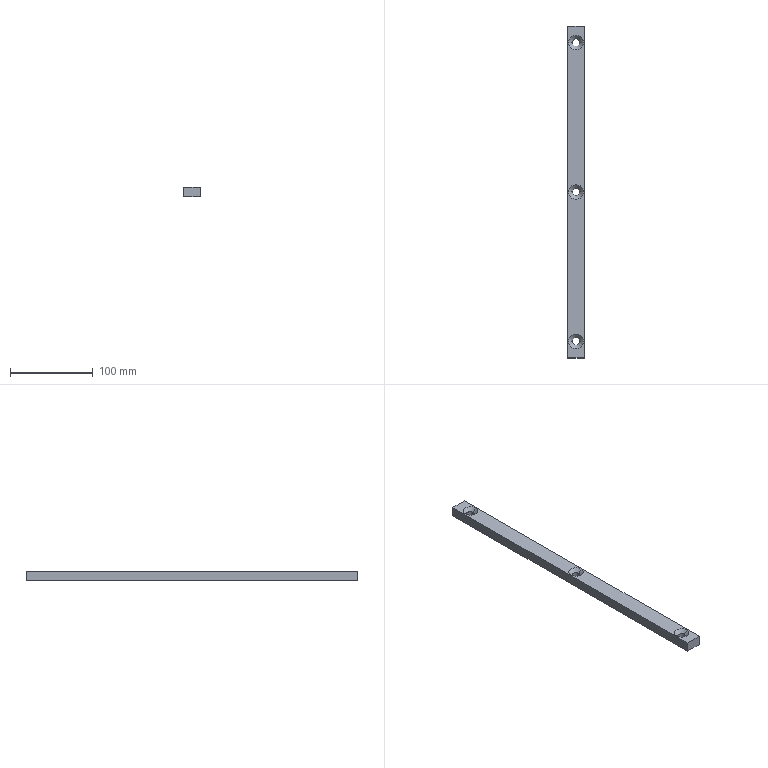Part | SolidWorks | features Extrusion 1, HoleWzd 1 | 1 solid | 18 faces | box 20 x 400 x 12 mm | volume 92676 mm3 | cone 6 | cylinder 6 | plane 6 | commonest cylinder face diameters 9 x6
STEP:
#1=CARTESIAN_POINT('',(5.5,380.,7.7));
#2=VERTEX_POINT('',#1);
#3=CARTESIAN_POINT('',(14.5,380.,7.7));
#4=VERTEX_POINT('',#3);
#5=CARTESIAN_POINT('',(10.,380.,7.7));
#6=DIRECTION('',(0.,0.,1.));
#7=DIRECTION('',(1.,0.,0.));
#8=AXIS2_PLACEMENT_3D('',#5,#6,#7);
#9=CIRCLE('',#8,4.5);
#10=EDGE_CURVE('',#2,#4,#9,.T.);
#11=ORIENTED_EDGE('',*,*,#10,.F.);
#12=CARTESIAN_POINT('',(1.2,380.,12.));
#13=VERTEX_POINT('',#12);
#14=CARTESIAN_POINT('',(1.2,380.,12.));
#15=DIRECTION('',(-0.7071,0.,0.7071));
#16=VECTOR('',#15,1000.);
#17=LINE('',#14,#16);
#18=EDGE_CURVE('',#2,#13,#17,.T.);
#19=ORIENTED_EDGE('',*,*,#18,.T.);
#20=CARTESIAN_POINT('',(18.8,380.,12.));
#21=VERTEX_POINT('',#20);
#22=CARTESIAN_POINT('',(10.,380.,12.));
#23=DIRECTION('',(0.,0.,1.));
#24=DIRECTION('',(1.,0.,0.));
#25=AXIS2_PLACEMENT_3D('',#22,#23,#24);
#26=CIRCLE('',#25,8.8);
#27=EDGE_CURVE('',#13,#21,#26,.T.);
#28=ORIENTED_EDGE('',*,*,#27,.T.);
#29=CARTESIAN_POINT('',(18.8,380.,12.));
#30=DIRECTION('',(0.7071,0.,0.7071));
#31=VECTOR('',#30,1000.);
#32=LINE('',#29,#31);
#33=EDGE_CURVE('',#4,#21,#32,.T.);
#34=ORIENTED_EDGE('',*,*,#33,.F.);
#35=EDGE_LOOP('',(#11,#19,#28,#34));
#36=FACE_OUTER_BOUND('',#35,.T.);
#37=CARTESIAN_POINT('',(10.,380.,12.));
#38=DIRECTION('',(0.,0.,1.));
#39=DIRECTION('',(1.,0.,0.));
#40=AXIS2_PLACEMENT_3D('',#37,#38,#39);
#41=CONICAL_SURFACE('',#40,8.8,0.7854);
#42=ADVANCED_FACE('',(#36),#41,.F.);
#43=CARTESIAN_POINT('',(5.5,380.,0.));
#44=VERTEX_POINT('',#43);
#45=CARTESIAN_POINT('',(14.5,380.,0.));
#46=VERTEX_POINT('',#45);
#47=CARTESIAN_POINT('',(10.,380.,0.));
#48=DIRECTION('',(0.,0.,1.));
#49=DIRECTION('',(1.,0.,0.));
#50=AXIS2_PLACEMENT_3D('',#47,#48,#49);
#51=CIRCLE('',#50,4.5);
#52=EDGE_CURVE('',#44,#46,#51,.T.);
#53=ORIENTED_EDGE('',*,*,#52,.F.);
#54=CARTESIAN_POINT('',(5.5,380.,12.));
#55=DIRECTION('',(0.,0.,1.));
#56=VECTOR('',#55,1000.);
#57=LINE('',#54,#56);
#58=EDGE_CURVE('',#44,#2,#57,.T.);
#59=ORIENTED_EDGE('',*,*,#58,.T.);
#60=ORIENTED_EDGE('',*,*,#10,.T.);
#61=CARTESIAN_POINT('',(14.5,380.,12.));
#62=DIRECTION('',(0.,0.,1.));
#63=VECTOR('',#62,1000.);
#64=LINE('',#61,#63);
#65=EDGE_CURVE('',#46,#4,#64,.T.);
#66=ORIENTED_EDGE('',*,*,#65,.F.);
#67=EDGE_LOOP('',(#53,#59,#60,#66));
#68=FACE_OUTER_BOUND('',#67,.T.);
#69=CARTESIAN_POINT('',(10.,380.,12.));
#70=DIRECTION('',(0.,0.,1.));
#71=DIRECTION('',(1.,0.,0.));
#72=AXIS2_PLACEMENT_3D('',#69,#70,#71);
#73=CYLINDRICAL_SURFACE('',#72,4.5);
#74=ADVANCED_FACE('',(#68),#73,.F.);
#75=CARTESIAN_POINT('',(5.5,200.,7.7));
#76=VERTEX_POINT('',#75);
#77=CARTESIAN_POINT('',(14.5,200.,7.7));
#78=VERTEX_POINT('',#77);
#79=CARTESIAN_POINT('',(10.,200.,7.7));
#80=DIRECTION('',(0.,0.,1.));
#81=DIRECTION('',(1.,0.,0.));
#82=AXIS2_PLACEMENT_3D('',#79,#80,#81);
#83=CIRCLE('',#82,4.5);
#84=EDGE_CURVE('',#76,#78,#83,.T.);
#85=ORIENTED_EDGE('',*,*,#84,.F.);
#86=CARTESIAN_POINT('',(1.2,200.,12.));
#87=VERTEX_POINT('',#86);
#88=CARTESIAN_POINT('',(1.2,200.,12.));
#89=DIRECTION('',(-0.7071,0.,0.7071));
#90=VECTOR('',#89,1000.);
#91=LINE('',#88,#90);
#92=EDGE_CURVE('',#76,#87,#91,.T.);
#93=ORIENTED_EDGE('',*,*,#92,.T.);
#94=CARTESIAN_POINT('',(18.8,200.,12.));
#95=VERTEX_POINT('',#94);
#96=CARTESIAN_POINT('',(10.,200.,12.));
#97=DIRECTION('',(0.,0.,1.));
#98=DIRECTION('',(1.,0.,0.));
#99=AXIS2_PLACEMENT_3D('',#96,#97,#98);
#100=CIRCLE('',#99,8.8);
#101=EDGE_CURVE('',#87,#95,#100,.T.);
#102=ORIENTED_EDGE('',*,*,#101,.T.);
#103=CARTESIAN_POINT('',(18.8,200.,12.));
#104=DIRECTION('',(0.7071,0.,0.7071));
#105=VECTOR('',#104,1000.);
#106=LINE('',#103,#105);
#107=EDGE_CURVE('',#78,#95,#106,.T.);
#108=ORIENTED_EDGE('',*,*,#107,.F.);
#109=EDGE_LOOP('',(#85,#93,#102,#108));
#110=FACE_OUTER_BOUND('',#109,.T.);
#111=CARTESIAN_POINT('',(10.,200.,12.));
#112=DIRECTION('',(0.,0.,1.));
#113=DIRECTION('',(1.,0.,0.));
#114=AXIS2_PLACEMENT_3D('',#111,#112,#113);
#115=CONICAL_SURFACE('',#114,8.8,0.7854);
#116=ADVANCED_FACE('',(#110),#115,.F.);
#117=CARTESIAN_POINT('',(5.5,200.,0.));
#118=VERTEX_POINT('',#117);
#119=CARTESIAN_POINT('',(14.5,200.,0.));
#120=VERTEX_POINT('',#119);
#121=CARTESIAN_POINT('',(10.,200.,0.));
#122=DIRECTION('',(0.,0.,1.));
#123=DIRECTION('',(1.,0.,0.));
#124=AXIS2_PLACEMENT_3D('',#121,#122,#123);
#125=CIRCLE('',#124,4.5);
#126=EDGE_CURVE('',#118,#120,#125,.T.);
#127=ORIENTED_EDGE('',*,*,#126,.F.);
#128=CARTESIAN_POINT('',(5.5,200.,12.));
#129=DIRECTION('',(0.,0.,1.));
#130=VECTOR('',#129,1000.);
#131=LINE('',#128,#130);
#132=EDGE_CURVE('',#118,#76,#131,.T.);
#133=ORIENTED_EDGE('',*,*,#132,.T.);
#134=ORIENTED_EDGE('',*,*,#84,.T.);
#135=CARTESIAN_POINT('',(14.5,200.,12.));
#136=DIRECTION('',(0.,0.,1.));
#137=VECTOR('',#136,1000.);
#138=LINE('',#135,#137);
#139=EDGE_CURVE('',#120,#78,#138,.T.);
#140=ORIENTED_EDGE('',*,*,#139,.F.);
#141=EDGE_LOOP('',(#127,#133,#134,#140));
#142=FACE_OUTER_BOUND('',#141,.T.);
#143=CARTESIAN_POINT('',(10.,200.,12.));
#144=DIRECTION('',(0.,0.,1.));
#145=DIRECTION('',(1.,0.,0.));
#146=AXIS2_PLACEMENT_3D('',#143,#144,#145);
#147=CYLINDRICAL_SURFACE('',#146,4.5);
#148=ADVANCED_FACE('',(#142),#147,.F.);
#149=CARTESIAN_POINT('',(5.5,20.,7.7));
#150=VERTEX_POINT('',#149);
#151=CARTESIAN_POINT('',(14.5,20.,7.7));
#152=VERTEX_POINT('',#151);
#153=CARTESIAN_POINT('',(10.,20.,7.7));
#154=DIRECTION('',(0.,0.,1.));
#155=DIRECTION('',(1.,0.,0.));
#156=AXIS2_PLACEMENT_3D('',#153,#154,#155);
#157=CIRCLE('',#156,4.5);
#158=EDGE_CURVE('',#150,#152,#157,.T.);
#159=ORIENTED_EDGE('',*,*,#158,.F.);
#160=CARTESIAN_POINT('',(1.2,20.,12.));
#161=VERTEX_POINT('',#160);
#162=CARTESIAN_POINT('',(1.2,20.,12.));
#163=DIRECTION('',(-0.7071,0.,0.7071));
#164=VECTOR('',#163,1000.);
#165=LINE('',#162,#164);
#166=EDGE_CURVE('',#150,#161,#165,.T.);
#167=ORIENTED_EDGE('',*,*,#166,.T.);
#168=CARTESIAN_POINT('',(18.8,20.,12.));
#169=VERTEX_POINT('',#168);
#170=CARTESIAN_POINT('',(10.,20.,12.));
#171=DIRECTION('',(0.,0.,1.));
#172=DIRECTION('',(1.,0.,0.));
#173=AXIS2_PLACEMENT_3D('',#170,#171,#172);
#174=CIRCLE('',#173,8.8);
#175=EDGE_CURVE('',#161,#169,#174,.T.);
#176=ORIENTED_EDGE('',*,*,#175,.T.);
#177=CARTESIAN_POINT('',(18.8,20.,12.));
#178=DIRECTION('',(0.7071,0.,0.7071));
#179=VECTOR('',#178,1000.);
#180=LINE('',#177,#179);
#181=EDGE_CURVE('',#152,#169,#180,.T.);
#182=ORIENTED_EDGE('',*,*,#181,.F.);
#183=EDGE_LOOP('',(#159,#167,#176,#182));
#184=FACE_OUTER_BOUND('',#183,.T.);
#185=CARTESIAN_POINT('',(10.,20.,12.));
#186=DIRECTION('',(0.,0.,1.));
#187=DIRECTION('',(1.,0.,0.));
#188=AXIS2_PLACEMENT_3D('',#185,#186,#187);
#189=CONICAL_SURFACE('',#188,8.8,0.7854);
#190=ADVANCED_FACE('',(#184),#189,.F.);
#191=CARTESIAN_POINT('',(5.5,20.,0.));
#192=VERTEX_POINT('',#191);
#193=CARTESIAN_POINT('',(14.5,20.,0.));
#194=VERTEX_POINT('',#193);
#195=CARTESIAN_POINT('',(10.,20.,0.));
#196=DIRECTION('',(0.,0.,1.));
#197=DIRECTION('',(1.,0.,0.));
#198=AXIS2_PLACEMENT_3D('',#195,#196,#197);
#199=CIRCLE('',#198,4.5);
#200=EDGE_CURVE('',#192,#194,#199,.T.);
#201=ORIENTED_EDGE('',*,*,#200,.F.);
#202=CARTESIAN_POINT('',(5.5,20.,12.));
#203=DIRECTION('',(0.,0.,1.));
#204=VECTOR('',#203,1000.);
#205=LINE('',#202,#204);
#206=EDGE_CURVE('',#192,#150,#205,.T.);
#207=ORIENTED_EDGE('',*,*,#206,.T.);
#208=ORIENTED_EDGE('',*,*,#158,.T.);
#209=CARTESIAN_POINT('',(14.5,20.,12.));
#210=DIRECTION('',(0.,0.,1.));
#211=VECTOR('',#210,1000.);
#212=LINE('',#209,#211);
#213=EDGE_CURVE('',#194,#152,#212,.T.);
#214=ORIENTED_EDGE('',*,*,#213,.F.);
#215=EDGE_LOOP('',(#201,#207,#208,#214));
#216=FACE_OUTER_BOUND('',#215,.T.);
#217=CARTESIAN_POINT('',(10.,20.,12.));
#218=DIRECTION('',(0.,0.,1.));
#219=DIRECTION('',(1.,0.,0.));
#220=AXIS2_PLACEMENT_3D('',#217,#218,#219);
#221=CYLINDRICAL_SURFACE('',#220,4.5);
#222=ADVANCED_FACE('',(#216),#221,.F.);
#223=CARTESIAN_POINT('',(0.,400.,0.));
#224=VERTEX_POINT('',#223);
#225=CARTESIAN_POINT('',(0.,0.,0.));
#226=VERTEX_POINT('',#225);
#227=CARTESIAN_POINT('',(0.,0.,0.));
#228=DIRECTION('',(0.,-1.,0.));
#229=VECTOR('',#228,1000.);
#230=LINE('',#227,#229);
#231=EDGE_CURVE('',#224,#226,#230,.T.);
#232=ORIENTED_EDGE('',*,*,#231,.T.);
#233=CARTESIAN_POINT('',(0.,0.,12.));
#234=VERTEX_POINT('',#233);
#235=CARTESIAN_POINT('',(0.,0.,12.));
#236=DIRECTION('',(0.,0.,-1.));
#237=VECTOR('',#236,1000.);
#238=LINE('',#235,#237);
#239=EDGE_CURVE('',#234,#226,#238,.T.);
#240=ORIENTED_EDGE('',*,*,#239,.F.);
#241=CARTESIAN_POINT('',(0.,400.,12.));
#242=VERTEX_POINT('',#241);
#243=CARTESIAN_POINT('',(0.,0.,12.));
#244=DIRECTION('',(0.,-1.,0.));
#245=VECTOR('',#244,1000.);
#246=LINE('',#243,#245);
#247=EDGE_CURVE('',#242,#234,#246,.T.);
#248=ORIENTED_EDGE('',*,*,#247,.F.);
#249=CARTESIAN_POINT('',(0.,400.,12.));
#250=DIRECTION('',(0.,0.,-1.));
#251=VECTOR('',#250,1000.);
#252=LINE('',#249,#251);
#253=EDGE_CURVE('',#242,#224,#252,.T.);
#254=ORIENTED_EDGE('',*,*,#253,.T.);
#255=EDGE_LOOP('',(#232,#240,#248,#254));
#256=FACE_OUTER_BOUND('',#255,.T.);
#257=CARTESIAN_POINT('',(0.,0.,12.));
#258=DIRECTION('',(1.,0.,0.));
#259=DIRECTION('',(0.,0.,-1.));
#260=AXIS2_PLACEMENT_3D('',#257,#258,#259);
#261=PLANE('',#260);
#262=ADVANCED_FACE('',(#256),#261,.F.);
#263=CARTESIAN_POINT('',(20.,0.,0.));
#264=VERTEX_POINT('',#263);
#265=CARTESIAN_POINT('',(0.,0.,0.));
#266=DIRECTION('',(1.,0.,0.));
#267=VECTOR('',#266,1000.);
#268=LINE('',#265,#267);
#269=EDGE_CURVE('',#226,#264,#268,.T.);
#270=ORIENTED_EDGE('',*,*,#269,.T.);
#271=CARTESIAN_POINT('',(20.,0.,12.));
#272=VERTEX_POINT('',#271);
#273=CARTESIAN_POINT('',(20.,0.,12.));
#274=DIRECTION('',(0.,0.,-1.));
#275=VECTOR('',#274,1000.);
#276=LINE('',#273,#275);
#277=EDGE_CURVE('',#272,#264,#276,.T.);
#278=ORIENTED_EDGE('',*,*,#277,.F.);
#279=CARTESIAN_POINT('',(0.,0.,12.));
#280=DIRECTION('',(1.,0.,0.));
#281=VECTOR('',#280,1000.);
#282=LINE('',#279,#281);
#283=EDGE_CURVE('',#234,#272,#282,.T.);
#284=ORIENTED_EDGE('',*,*,#283,.F.);
#285=ORIENTED_EDGE('',*,*,#239,.T.);
#286=EDGE_LOOP('',(#270,#278,#284,#285));
#287=FACE_OUTER_BOUND('',#286,.T.);
#288=CARTESIAN_POINT('',(0.,0.,12.));
#289=DIRECTION('',(0.,1.,0.));
#290=DIRECTION('',(0.,0.,1.));
#291=AXIS2_PLACEMENT_3D('',#288,#289,#290);
#292=PLANE('',#291);
#293=ADVANCED_FACE('',(#287),#292,.F.);
#294=CARTESIAN_POINT('',(20.,400.,0.));
#295=VERTEX_POINT('',#294);
#296=CARTESIAN_POINT('',(20.,0.,0.));
#297=DIRECTION('',(0.,1.,0.));
#298=VECTOR('',#297,1000.);
#299=LINE('',#296,#298);
#300=EDGE_CURVE('',#264,#295,#299,.T.);
#301=ORIENTED_EDGE('',*,*,#300,.T.);
#302=CARTESIAN_POINT('',(20.,400.,12.));
#303=VERTEX_POINT('',#302);
#304=CARTESIAN_POINT('',(20.,400.,12.));
#305=DIRECTION('',(0.,0.,-1.));
#306=VECTOR('',#305,1000.);
#307=LINE('',#304,#306);
#308=EDGE_CURVE('',#303,#295,#307,.T.);
#309=ORIENTED_EDGE('',*,*,#308,.F.);
#310=CARTESIAN_POINT('',(20.,0.,12.));
#311=DIRECTION('',(0.,1.,0.));
#312=VECTOR('',#311,1000.);
#313=LINE('',#310,#312);
#314=EDGE_CURVE('',#272,#303,#313,.T.);
#315=ORIENTED_EDGE('',*,*,#314,.F.);
#316=ORIENTED_EDGE('',*,*,#277,.T.);
#317=EDGE_LOOP('',(#301,#309,#315,#316));
#318=FACE_OUTER_BOUND('',#317,.T.);
#319=CARTESIAN_POINT('',(20.,0.,12.));
#320=DIRECTION('',(-1.,0.,0.));
#321=DIRECTION('',(0.,0.,1.));
#322=AXIS2_PLACEMENT_3D('',#319,#320,#321);
#323=PLANE('',#322);
#324=ADVANCED_FACE('',(#318),#323,.F.);
#325=CARTESIAN_POINT('',(0.,400.,0.));
#326=DIRECTION('',(-1.,0.,0.));
#327=VECTOR('',#326,1000.);
#328=LINE('',#325,#327);
#329=EDGE_CURVE('',#295,#224,#328,.T.);
#330=ORIENTED_EDGE('',*,*,#329,.T.);
#331=ORIENTED_EDGE('',*,*,#253,.F.);
#332=CARTESIAN_POINT('',(0.,400.,12.));
#333=DIRECTION('',(-1.,0.,0.));
#334=VECTOR('',#333,1000.);
#335=LINE('',#332,#334);
#336=EDGE_CURVE('',#303,#242,#335,.T.);
#337=ORIENTED_EDGE('',*,*,#336,.F.);
#338=ORIENTED_EDGE('',*,*,#308,.T.);
#339=EDGE_LOOP('',(#330,#331,#337,#338));
#340=FACE_OUTER_BOUND('',#339,.T.);
#341=CARTESIAN_POINT('',(0.,400.,12.));
#342=DIRECTION('',(0.,-1.,0.));
#343=DIRECTION('',(0.,0.,-1.));
#344=AXIS2_PLACEMENT_3D('',#341,#342,#343);
#345=PLANE('',#344);
#346=ADVANCED_FACE('',(#340),#345,.F.);
#347=CARTESIAN_POINT('',(10.,380.,12.));
#348=DIRECTION('',(0.,0.,1.));
#349=DIRECTION('',(1.,0.,0.));
#350=AXIS2_PLACEMENT_3D('',#347,#348,#349);
#351=CIRCLE('',#350,8.8);
#352=EDGE_CURVE('',#21,#13,#351,.T.);
#353=ORIENTED_EDGE('',*,*,#352,.F.);
#354=ORIENTED_EDGE('',*,*,#27,.F.);
#355=EDGE_LOOP('',(#353,#354));
#356=FACE_BOUND('',#355,.T.);
#357=CARTESIAN_POINT('',(10.,200.,12.));
#358=DIRECTION('',(0.,0.,1.));
#359=DIRECTION('',(1.,0.,0.));
#360=AXIS2_PLACEMENT_3D('',#357,#358,#359);
#361=CIRCLE('',#360,8.8);
#362=EDGE_CURVE('',#95,#87,#361,.T.);
#363=ORIENTED_EDGE('',*,*,#362,.F.);
#364=ORIENTED_EDGE('',*,*,#101,.F.);
#365=EDGE_LOOP('',(#363,#364));
#366=FACE_BOUND('',#365,.T.);
#367=CARTESIAN_POINT('',(10.,20.,12.));
#368=DIRECTION('',(0.,0.,1.));
#369=DIRECTION('',(1.,0.,0.));
#370=AXIS2_PLACEMENT_3D('',#367,#368,#369);
#371=CIRCLE('',#370,8.8);
#372=EDGE_CURVE('',#169,#161,#371,.T.);
#373=ORIENTED_EDGE('',*,*,#372,.F.);
#374=ORIENTED_EDGE('',*,*,#175,.F.);
#375=EDGE_LOOP('',(#373,#374));
#376=FACE_BOUND('',#375,.T.);
#377=ORIENTED_EDGE('',*,*,#247,.T.);
#378=ORIENTED_EDGE('',*,*,#283,.T.);
#379=ORIENTED_EDGE('',*,*,#314,.T.);
#380=ORIENTED_EDGE('',*,*,#336,.T.);
#381=EDGE_LOOP('',(#377,#378,#379,#380));
#382=FACE_OUTER_BOUND('',#381,.T.);
#383=CARTESIAN_POINT('',(0.,0.,12.));
#384=DIRECTION('',(0.,0.,-1.));
#385=DIRECTION('',(-1.,0.,0.));
#386=AXIS2_PLACEMENT_3D('',#383,#384,#385);
#387=PLANE('',#386);
#388=ADVANCED_FACE('',(#356,#366,#376,#382),#387,.F.);
#389=CARTESIAN_POINT('',(10.,380.,0.));
#390=DIRECTION('',(0.,0.,1.));
#391=DIRECTION('',(1.,0.,0.));
#392=AXIS2_PLACEMENT_3D('',#389,#390,#391);
#393=CIRCLE('',#392,4.5);
#394=EDGE_CURVE('',#46,#44,#393,.T.);
#395=ORIENTED_EDGE('',*,*,#394,.T.);
#396=ORIENTED_EDGE('',*,*,#52,.T.);
#397=EDGE_LOOP('',(#395,#396));
#398=FACE_BOUND('',#397,.T.);
#399=CARTESIAN_POINT('',(10.,200.,0.));
#400=DIRECTION('',(0.,0.,1.));
#401=DIRECTION('',(1.,0.,0.));
#402=AXIS2_PLACEMENT_3D('',#399,#400,#401);
#403=CIRCLE('',#402,4.5);
#404=EDGE_CURVE('',#120,#118,#403,.T.);
#405=ORIENTED_EDGE('',*,*,#404,.T.);
#406=ORIENTED_EDGE('',*,*,#126,.T.);
#407=EDGE_LOOP('',(#405,#406));
#408=FACE_BOUND('',#407,.T.);
#409=CARTESIAN_POINT('',(10.,20.,0.));
#410=DIRECTION('',(0.,0.,1.));
#411=DIRECTION('',(1.,0.,0.));
#412=AXIS2_PLACEMENT_3D('',#409,#410,#411);
#413=CIRCLE('',#412,4.5);
#414=EDGE_CURVE('',#194,#192,#413,.T.);
#415=ORIENTED_EDGE('',*,*,#414,.T.);
#416=ORIENTED_EDGE('',*,*,#200,.T.);
#417=EDGE_LOOP('',(#415,#416));
#418=FACE_BOUND('',#417,.T.);
#419=ORIENTED_EDGE('',*,*,#231,.F.);
#420=ORIENTED_EDGE('',*,*,#329,.F.);
#421=ORIENTED_EDGE('',*,*,#300,.F.);
#422=ORIENTED_EDGE('',*,*,#269,.F.);
#423=EDGE_LOOP('',(#419,#420,#421,#422));
#424=FACE_OUTER_BOUND('',#423,.T.);
#425=CARTESIAN_POINT('',(0.,0.,0.));
#426=DIRECTION('',(0.,0.,-1.));
#427=DIRECTION('',(-1.,0.,0.));
#428=AXIS2_PLACEMENT_3D('',#425,#426,#427);
#429=PLANE('',#428);
#430=ADVANCED_FACE('',(#398,#408,#418,#424),#429,.T.);
#431=ORIENTED_EDGE('',*,*,#206,.F.);
#432=ORIENTED_EDGE('',*,*,#414,.F.);
#433=ORIENTED_EDGE('',*,*,#213,.T.);
#434=CARTESIAN_POINT('',(10.,20.,7.7));
#435=DIRECTION('',(0.,0.,1.));
#436=DIRECTION('',(1.,0.,0.));
#437=AXIS2_PLACEMENT_3D('',#434,#435,#436);
#438=CIRCLE('',#437,4.5);
#439=EDGE_CURVE('',#152,#150,#438,.T.);
#440=ORIENTED_EDGE('',*,*,#439,.T.);
#441=EDGE_LOOP('',(#431,#432,#433,#440));
#442=FACE_OUTER_BOUND('',#441,.T.);
#443=CARTESIAN_POINT('',(10.,20.,12.));
#444=DIRECTION('',(0.,0.,1.));
#445=DIRECTION('',(1.,0.,0.));
#446=AXIS2_PLACEMENT_3D('',#443,#444,#445);
#447=CYLINDRICAL_SURFACE('',#446,4.5);
#448=ADVANCED_FACE('',(#442),#447,.F.);
#449=ORIENTED_EDGE('',*,*,#166,.F.);
#450=ORIENTED_EDGE('',*,*,#439,.F.);
#451=ORIENTED_EDGE('',*,*,#181,.T.);
#452=ORIENTED_EDGE('',*,*,#372,.T.);
#453=EDGE_LOOP('',(#449,#450,#451,#452));
#454=FACE_OUTER_BOUND('',#453,.T.);
#455=CARTESIAN_POINT('',(10.,20.,12.));
#456=DIRECTION('',(0.,0.,1.));
#457=DIRECTION('',(1.,0.,0.));
#458=AXIS2_PLACEMENT_3D('',#455,#456,#457);
#459=CONICAL_SURFACE('',#458,8.8,0.7854);
#460=ADVANCED_FACE('',(#454),#459,.F.);
#461=ORIENTED_EDGE('',*,*,#132,.F.);
#462=ORIENTED_EDGE('',*,*,#404,.F.);
#463=ORIENTED_EDGE('',*,*,#139,.T.);
#464=CARTESIAN_POINT('',(10.,200.,7.7));
#465=DIRECTION('',(0.,0.,1.));
#466=DIRECTION('',(1.,0.,0.));
#467=AXIS2_PLACEMENT_3D('',#464,#465,#466);
#468=CIRCLE('',#467,4.5);
#469=EDGE_CURVE('',#78,#76,#468,.T.);
#470=ORIENTED_EDGE('',*,*,#469,.T.);
#471=EDGE_LOOP('',(#461,#462,#463,#470));
#472=FACE_OUTER_BOUND('',#471,.T.);
#473=CARTESIAN_POINT('',(10.,200.,12.));
#474=DIRECTION('',(0.,0.,1.));
#475=DIRECTION('',(1.,0.,0.));
#476=AXIS2_PLACEMENT_3D('',#473,#474,#475);
#477=CYLINDRICAL_SURFACE('',#476,4.5);
#478=ADVANCED_FACE('',(#472),#477,.F.);
#479=ORIENTED_EDGE('',*,*,#92,.F.);
#480=ORIENTED_EDGE('',*,*,#469,.F.);
#481=ORIENTED_EDGE('',*,*,#107,.T.);
#482=ORIENTED_EDGE('',*,*,#362,.T.);
#483=EDGE_LOOP('',(#479,#480,#481,#482));
#484=FACE_OUTER_BOUND('',#483,.T.);
#485=CARTESIAN_POINT('',(10.,200.,12.));
#486=DIRECTION('',(0.,0.,1.));
#487=DIRECTION('',(1.,0.,0.));
#488=AXIS2_PLACEMENT_3D('',#485,#486,#487);
#489=CONICAL_SURFACE('',#488,8.8,0.7854);
#490=ADVANCED_FACE('',(#484),#489,.F.);
#491=ORIENTED_EDGE('',*,*,#58,.F.);
#492=ORIENTED_EDGE('',*,*,#394,.F.);
#493=ORIENTED_EDGE('',*,*,#65,.T.);
#494=CARTESIAN_POINT('',(10.,380.,7.7));
#495=DIRECTION('',(0.,0.,1.));
#496=DIRECTION('',(1.,0.,0.));
#497=AXIS2_PLACEMENT_3D('',#494,#495,#496);
#498=CIRCLE('',#497,4.5);
#499=EDGE_CURVE('',#4,#2,#498,.T.);
#500=ORIENTED_EDGE('',*,*,#499,.T.);
#501=EDGE_LOOP('',(#491,#492,#493,#500));
#502=FACE_OUTER_BOUND('',#501,.T.);
#503=CARTESIAN_POINT('',(10.,380.,12.));
#504=DIRECTION('',(0.,0.,1.));
#505=DIRECTION('',(1.,0.,0.));
#506=AXIS2_PLACEMENT_3D('',#503,#504,#505);
#507=CYLINDRICAL_SURFACE('',#506,4.5);
#508=ADVANCED_FACE('',(#502),#507,.F.);
#509=ORIENTED_EDGE('',*,*,#18,.F.);
#510=ORIENTED_EDGE('',*,*,#499,.F.);
#511=ORIENTED_EDGE('',*,*,#33,.T.);
#512=ORIENTED_EDGE('',*,*,#352,.T.);
#513=EDGE_LOOP('',(#509,#510,#511,#512));
#514=FACE_OUTER_BOUND('',#513,.T.);
#515=CARTESIAN_POINT('',(10.,380.,12.));
#516=DIRECTION('',(0.,0.,1.));
#517=DIRECTION('',(1.,0.,0.));
#518=AXIS2_PLACEMENT_3D('',#515,#516,#517);
#519=CONICAL_SURFACE('',#518,8.8,0.7854);
#520=ADVANCED_FACE('',(#514),#519,.F.);
#521=CLOSED_SHELL('',(#42,#74,#116,#148,#190,#222,#262,#293,#324,#346,#388,#430,#448,#460,#478,#490,#508,#520));
#522=MANIFOLD_SOLID_BREP('',#521);
#523=CARTESIAN_POINT('',(0.,0.,0.));
#524=DIRECTION('',(0.,0.,1.));
#525=DIRECTION('',(1.,0.,0.));
#526=AXIS2_PLACEMENT_3D('',#523,#524,#525);
#527=(LENGTH_UNIT()NAMED_UNIT(*)SI_UNIT(.MILLI.,.METRE.));
#528=UNCERTAINTY_MEASURE_WITH_UNIT(LENGTH_MEASURE(0.00001),#527,'','');
#529=(NAMED_UNIT(*)PLANE_ANGLE_UNIT()SI_UNIT($,.RADIAN.));
#530=(NAMED_UNIT(*)SI_UNIT($,.STERADIAN.)SOLID_ANGLE_UNIT());
#531=(GEOMETRIC_REPRESENTATION_CONTEXT(3)GLOBAL_UNCERTAINTY_ASSIGNED_CONTEXT((#528))GLOBAL_UNIT_ASSIGNED_CONTEXT((#527,#529,#530))REPRESENTATION_CONTEXT('',''));
#532=ADVANCED_BREP_SHAPE_REPRESENTATION('',(#522,#526),#531);